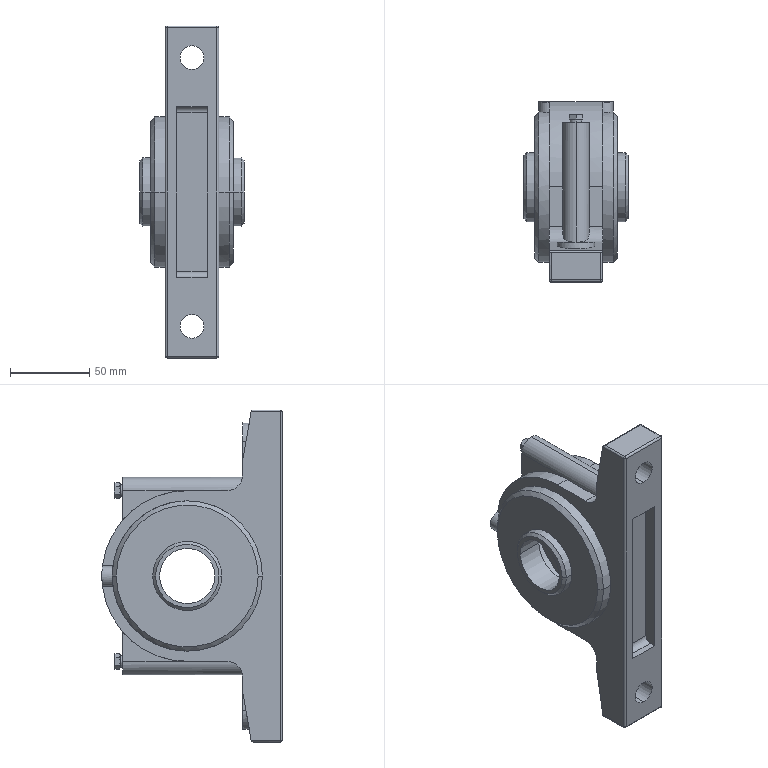Part | SolidWorks | features BaseBody 1 | 1 solid | 141 faces | box 66 x 114 x 210 mm | volume 426890 mm3 | plane 52 | cylinder 49 | cone 36 | spline 4 | commonest cylinder face diameters 2.4 x10 7.2 x4 15 x4 35 x4 43.75 x4 69.231 x4